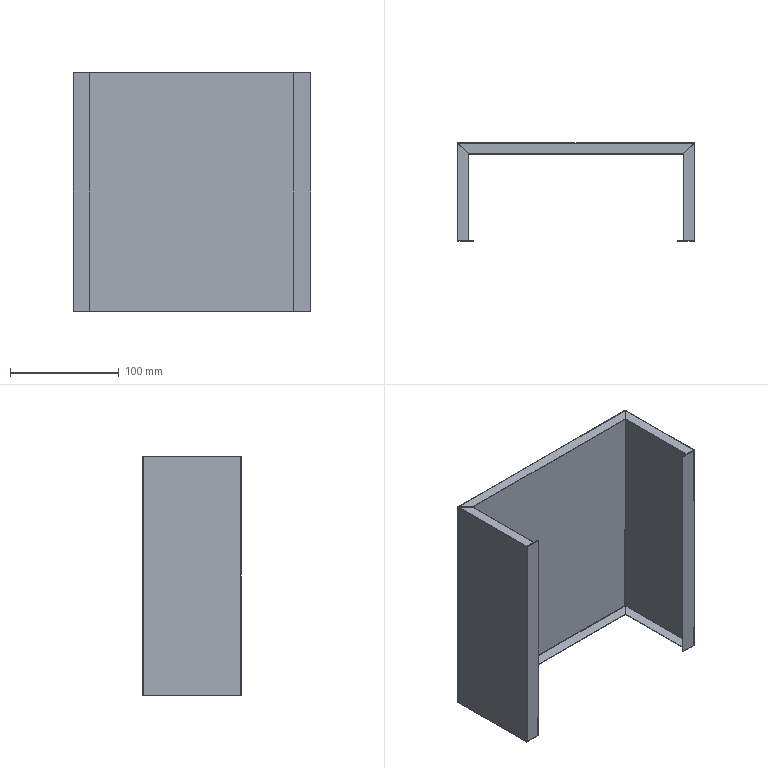Part | SolidWorks | features EdgeFlange 2, FlatPattern 1, SMBaseFlange 1, SheetMetal 1, UnFold 1 | 1 solid | 94 faces | box 218 x 90 x 220 mm | volume 50340 mm3 | plane 58 | cylinder 20 | spline 16 | commonest cylinder face diameters 0.2 x10 1.2 x10